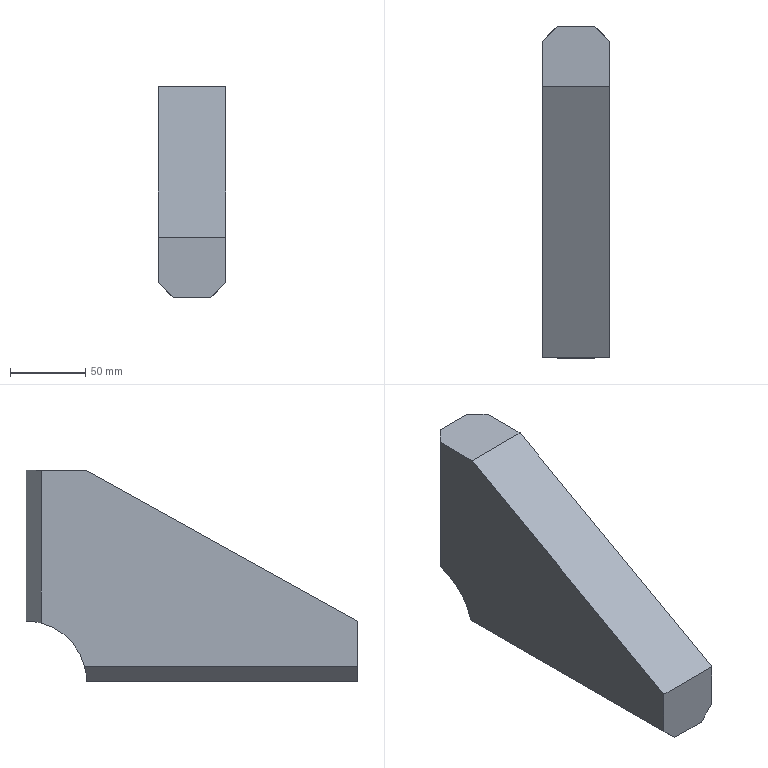Part | SolidWorks | features Chamfer 1, Extrusion 1 | 1 solid | 12 faces | box 45 x 220 x 140 mm | volume 896409 mm3 | plane 11 | cylinder 1 | commonest cylinder face diameters 80 x1
STEP:
#1=CARTESIAN_POINT('',(-22.5,0.,40.));
#2=VERTEX_POINT('',#1);
#3=CARTESIAN_POINT('',(-22.5,0.,10.));
#4=VERTEX_POINT('',#3);
#5=CARTESIAN_POINT('',(-22.5,0.,40.));
#6=DIRECTION('',(0.,0.,-1.));
#7=VECTOR('',#6,1000.);
#8=LINE('',#5,#7);
#9=EDGE_CURVE('',#2,#4,#8,.T.);
#10=ORIENTED_EDGE('',*,*,#9,.T.);
#11=CARTESIAN_POINT('',(-12.5,0.,0.));
#12=VERTEX_POINT('',#11);
#13=CARTESIAN_POINT('',(-12.5,0.,0.));
#14=DIRECTION('',(0.7071,0.,-0.7071));
#15=VECTOR('',#14,1000.);
#16=LINE('',#13,#15);
#17=EDGE_CURVE('',#4,#12,#16,.T.);
#18=ORIENTED_EDGE('',*,*,#17,.T.);
#19=CARTESIAN_POINT('',(12.5,0.,0.));
#20=VERTEX_POINT('',#19);
#21=CARTESIAN_POINT('',(22.5,0.,0.));
#22=DIRECTION('',(-1.,0.,0.));
#23=VECTOR('',#22,1000.);
#24=LINE('',#21,#23);
#25=EDGE_CURVE('',#20,#12,#24,.T.);
#26=ORIENTED_EDGE('',*,*,#25,.F.);
#27=CARTESIAN_POINT('',(22.5,0.,10.));
#28=VERTEX_POINT('',#27);
#29=CARTESIAN_POINT('',(22.5,0.,10.));
#30=DIRECTION('',(0.7071,0.,0.7071));
#31=VECTOR('',#30,1000.);
#32=LINE('',#29,#31);
#33=EDGE_CURVE('',#20,#28,#32,.T.);
#34=ORIENTED_EDGE('',*,*,#33,.T.);
#35=CARTESIAN_POINT('',(22.5,0.,40.));
#36=VERTEX_POINT('',#35);
#37=CARTESIAN_POINT('',(22.5,0.,40.));
#38=DIRECTION('',(0.,0.,-1.));
#39=VECTOR('',#38,1000.);
#40=LINE('',#37,#39);
#41=EDGE_CURVE('',#36,#28,#40,.T.);
#42=ORIENTED_EDGE('',*,*,#41,.F.);
#43=CARTESIAN_POINT('',(22.5,0.,40.));
#44=DIRECTION('',(-1.,0.,0.));
#45=VECTOR('',#44,1000.);
#46=LINE('',#43,#45);
#47=EDGE_CURVE('',#36,#2,#46,.T.);
#48=ORIENTED_EDGE('',*,*,#47,.T.);
#49=EDGE_LOOP('',(#10,#18,#26,#34,#42,#48));
#50=FACE_OUTER_BOUND('',#49,.T.);
#51=CARTESIAN_POINT('',(22.5,0.,40.));
#52=DIRECTION('',(0.,1.,0.));
#53=DIRECTION('',(0.,0.,1.));
#54=AXIS2_PLACEMENT_3D('',#51,#52,#53);
#55=PLANE('',#54);
#56=ADVANCED_FACE('',(#50),#55,.F.);
#57=ORIENTED_EDGE('',*,*,#25,.T.);
#58=CARTESIAN_POINT('',(-12.5,180.,0.));
#59=VERTEX_POINT('',#58);
#60=CARTESIAN_POINT('',(-12.5,0.,0.));
#61=DIRECTION('',(0.,1.,0.));
#62=VECTOR('',#61,1000.);
#63=LINE('',#60,#62);
#64=EDGE_CURVE('',#12,#59,#63,.T.);
#65=ORIENTED_EDGE('',*,*,#64,.T.);
#66=CARTESIAN_POINT('',(12.5,180.,0.));
#67=VERTEX_POINT('',#66);
#68=CARTESIAN_POINT('',(22.5,180.,0.));
#69=DIRECTION('',(-1.,0.,0.));
#70=VECTOR('',#69,1000.);
#71=LINE('',#68,#70);
#72=EDGE_CURVE('',#67,#59,#71,.T.);
#73=ORIENTED_EDGE('',*,*,#72,.F.);
#74=CARTESIAN_POINT('',(12.5,0.,0.));
#75=DIRECTION('',(0.,-1.,0.));
#76=VECTOR('',#75,1000.);
#77=LINE('',#74,#76);
#78=EDGE_CURVE('',#67,#20,#77,.T.);
#79=ORIENTED_EDGE('',*,*,#78,.T.);
#80=EDGE_LOOP('',(#57,#65,#73,#79));
#81=FACE_OUTER_BOUND('',#80,.T.);
#82=CARTESIAN_POINT('',(22.5,0.,0.));
#83=DIRECTION('',(0.,0.,1.));
#84=DIRECTION('',(1.,0.,0.));
#85=AXIS2_PLACEMENT_3D('',#82,#83,#84);
#86=PLANE('',#85);
#87=ADVANCED_FACE('',(#81),#86,.F.);
#88=CARTESIAN_POINT('',(12.5,220.,40.));
#89=VERTEX_POINT('',#88);
#90=CARTESIAN_POINT('',(-12.5,220.,40.));
#91=VERTEX_POINT('',#90);
#92=CARTESIAN_POINT('',(22.5,220.,40.));
#93=DIRECTION('',(-1.,0.,0.));
#94=VECTOR('',#93,1000.);
#95=LINE('',#92,#94);
#96=EDGE_CURVE('',#89,#91,#95,.T.);
#97=ORIENTED_EDGE('',*,*,#96,.F.);
#98=CARTESIAN_POINT('',(22.5,210.,38.73));
#99=VERTEX_POINT('',#98);
#100=CARTESIAN_POINT('',(12.5,220.,40.));
#101=CARTESIAN_POINT('',(15.878,216.622,40.));
#102=CARTESIAN_POINT('',(19.229,213.271,39.574));
#103=CARTESIAN_POINT('',(22.5,210.,38.73));
#104=(BOUNDED_CURVE()B_SPLINE_CURVE(3,(#100,#101,#102,#103),.UNSPECIFIED.,.F.,.F.)B_SPLINE_CURVE_WITH_KNOTS((4,4),(1.571,1.823),.UNSPECIFIED.)CURVE()GEOMETRIC_REPRESENTATION_ITEM()RATIONAL_B_SPLINE_CURVE((1.,0.9947,0.9947,1.))REPRESENTATION_ITEM(''));
#105=EDGE_CURVE('',#89,#99,#104,.T.);
#106=ORIENTED_EDGE('',*,*,#105,.T.);
#107=CARTESIAN_POINT('',(22.5,181.27,10.));
#108=VERTEX_POINT('',#107);
#109=CARTESIAN_POINT('',(22.5,220.,0.));
#110=DIRECTION('',(-1.,0.,0.));
#111=DIRECTION('',(0.,0.,-1.));
#112=AXIS2_PLACEMENT_3D('',#109,#110,#111);
#113=CIRCLE('',#112,40.);
#114=EDGE_CURVE('',#108,#99,#113,.T.);
#115=ORIENTED_EDGE('',*,*,#114,.F.);
#116=CARTESIAN_POINT('',(22.5,181.27,10.));
#117=CARTESIAN_POINT('',(19.229,180.426,6.729));
#118=CARTESIAN_POINT('',(15.878,180.,3.378));
#119=CARTESIAN_POINT('',(12.5,180.,0.));
#120=(BOUNDED_CURVE()B_SPLINE_CURVE(3,(#116,#117,#118,#119),.UNSPECIFIED.,.F.,.F.)B_SPLINE_CURVE_WITH_KNOTS((4,4),(4.46,4.712),.UNSPECIFIED.)CURVE()GEOMETRIC_REPRESENTATION_ITEM()RATIONAL_B_SPLINE_CURVE((1.,0.9947,0.9947,1.))REPRESENTATION_ITEM(''));
#121=EDGE_CURVE('',#108,#67,#120,.T.);
#122=ORIENTED_EDGE('',*,*,#121,.T.);
#123=ORIENTED_EDGE('',*,*,#72,.T.);
#124=CARTESIAN_POINT('',(-22.5,181.27,10.));
#125=VERTEX_POINT('',#124);
#126=CARTESIAN_POINT('',(-12.5,180.,0.));
#127=CARTESIAN_POINT('',(-15.878,180.,3.378));
#128=CARTESIAN_POINT('',(-19.229,180.426,6.729));
#129=CARTESIAN_POINT('',(-22.5,181.27,10.));
#130=(BOUNDED_CURVE()B_SPLINE_CURVE(3,(#126,#127,#128,#129),.UNSPECIFIED.,.F.,.F.)B_SPLINE_CURVE_WITH_KNOTS((4,4),(4.712,4.965),.UNSPECIFIED.)CURVE()GEOMETRIC_REPRESENTATION_ITEM()RATIONAL_B_SPLINE_CURVE((1.,0.9947,0.9947,1.))REPRESENTATION_ITEM(''));
#131=EDGE_CURVE('',#59,#125,#130,.T.);
#132=ORIENTED_EDGE('',*,*,#131,.T.);
#133=CARTESIAN_POINT('',(-22.5,210.,38.73));
#134=VERTEX_POINT('',#133);
#135=CARTESIAN_POINT('',(-22.5,220.,0.));
#136=DIRECTION('',(-1.,0.,0.));
#137=DIRECTION('',(0.,0.,-1.));
#138=AXIS2_PLACEMENT_3D('',#135,#136,#137);
#139=CIRCLE('',#138,40.);
#140=EDGE_CURVE('',#125,#134,#139,.T.);
#141=ORIENTED_EDGE('',*,*,#140,.T.);
#142=CARTESIAN_POINT('',(-22.5,210.,38.73));
#143=CARTESIAN_POINT('',(-19.229,213.271,39.574));
#144=CARTESIAN_POINT('',(-15.878,216.622,40.));
#145=CARTESIAN_POINT('',(-12.5,220.,40.));
#146=(BOUNDED_CURVE()B_SPLINE_CURVE(3,(#142,#143,#144,#145),.UNSPECIFIED.,.F.,.F.)B_SPLINE_CURVE_WITH_KNOTS((4,4),(1.318,1.571),.UNSPECIFIED.)CURVE()GEOMETRIC_REPRESENTATION_ITEM()RATIONAL_B_SPLINE_CURVE((1.,0.9947,0.9947,1.))REPRESENTATION_ITEM(''));
#147=EDGE_CURVE('',#134,#91,#146,.T.);
#148=ORIENTED_EDGE('',*,*,#147,.T.);
#149=EDGE_LOOP('',(#97,#106,#115,#122,#123,#132,#141,#148));
#150=FACE_OUTER_BOUND('',#149,.T.);
#151=CARTESIAN_POINT('',(22.5,220.,0.));
#152=DIRECTION('',(-1.,0.,0.));
#153=DIRECTION('',(0.,0.,1.));
#154=AXIS2_PLACEMENT_3D('',#151,#152,#153);
#155=CYLINDRICAL_SURFACE('',#154,40.);
#156=ADVANCED_FACE('',(#150),#155,.F.);
#157=CARTESIAN_POINT('',(12.5,220.,140.));
#158=VERTEX_POINT('',#157);
#159=CARTESIAN_POINT('',(-12.5,220.,140.));
#160=VERTEX_POINT('',#159);
#161=CARTESIAN_POINT('',(22.5,220.,140.));
#162=DIRECTION('',(-1.,0.,0.));
#163=VECTOR('',#162,1000.);
#164=LINE('',#161,#163);
#165=EDGE_CURVE('',#158,#160,#164,.T.);
#166=ORIENTED_EDGE('',*,*,#165,.F.);
#167=CARTESIAN_POINT('',(12.5,220.,40.));
#168=DIRECTION('',(0.,0.,-1.));
#169=VECTOR('',#168,1000.);
#170=LINE('',#167,#169);
#171=EDGE_CURVE('',#158,#89,#170,.T.);
#172=ORIENTED_EDGE('',*,*,#171,.T.);
#173=ORIENTED_EDGE('',*,*,#96,.T.);
#174=CARTESIAN_POINT('',(-12.5,220.,40.));
#175=DIRECTION('',(0.,0.,1.));
#176=VECTOR('',#175,1000.);
#177=LINE('',#174,#176);
#178=EDGE_CURVE('',#91,#160,#177,.T.);
#179=ORIENTED_EDGE('',*,*,#178,.T.);
#180=EDGE_LOOP('',(#166,#172,#173,#179));
#181=FACE_OUTER_BOUND('',#180,.T.);
#182=CARTESIAN_POINT('',(22.5,220.,40.));
#183=DIRECTION('',(0.,-1.,0.));
#184=DIRECTION('',(0.,0.,-1.));
#185=AXIS2_PLACEMENT_3D('',#182,#183,#184);
#186=PLANE('',#185);
#187=ADVANCED_FACE('',(#181),#186,.F.);
#188=CARTESIAN_POINT('',(22.5,210.,140.));
#189=VERTEX_POINT('',#188);
#190=CARTESIAN_POINT('',(22.5,180.,140.));
#191=VERTEX_POINT('',#190);
#192=CARTESIAN_POINT('',(22.5,220.,140.));
#193=DIRECTION('',(0.,-1.,0.));
#194=VECTOR('',#193,1000.);
#195=LINE('',#192,#194);
#196=EDGE_CURVE('',#189,#191,#195,.T.);
#197=ORIENTED_EDGE('',*,*,#196,.F.);
#198=CARTESIAN_POINT('',(22.5,210.,140.));
#199=DIRECTION('',(-0.7071,0.7071,0.));
#200=VECTOR('',#199,1000.);
#201=LINE('',#198,#200);
#202=EDGE_CURVE('',#189,#158,#201,.T.);
#203=ORIENTED_EDGE('',*,*,#202,.T.);
#204=ORIENTED_EDGE('',*,*,#165,.T.);
#205=CARTESIAN_POINT('',(-22.5,210.,140.));
#206=VERTEX_POINT('',#205);
#207=CARTESIAN_POINT('',(-12.5,220.,140.));
#208=DIRECTION('',(-0.7071,-0.7071,0.));
#209=VECTOR('',#208,1000.);
#210=LINE('',#207,#209);
#211=EDGE_CURVE('',#160,#206,#210,.T.);
#212=ORIENTED_EDGE('',*,*,#211,.T.);
#213=CARTESIAN_POINT('',(-22.5,180.,140.));
#214=VERTEX_POINT('',#213);
#215=CARTESIAN_POINT('',(-22.5,220.,140.));
#216=DIRECTION('',(0.,-1.,0.));
#217=VECTOR('',#216,1000.);
#218=LINE('',#215,#217);
#219=EDGE_CURVE('',#206,#214,#218,.T.);
#220=ORIENTED_EDGE('',*,*,#219,.T.);
#221=CARTESIAN_POINT('',(22.5,180.,140.));
#222=DIRECTION('',(-1.,0.,0.));
#223=VECTOR('',#222,1000.);
#224=LINE('',#221,#223);
#225=EDGE_CURVE('',#191,#214,#224,.T.);
#226=ORIENTED_EDGE('',*,*,#225,.F.);
#227=EDGE_LOOP('',(#197,#203,#204,#212,#220,#226));
#228=FACE_OUTER_BOUND('',#227,.T.);
#229=CARTESIAN_POINT('',(22.5,220.,140.));
#230=DIRECTION('',(0.,0.,-1.));
#231=DIRECTION('',(-1.,0.,0.));
#232=AXIS2_PLACEMENT_3D('',#229,#230,#231);
#233=PLANE('',#232);
#234=ADVANCED_FACE('',(#228),#233,.F.);
#235=CARTESIAN_POINT('',(-22.5,180.,140.));
#236=DIRECTION('',(0.,-0.8742,-0.4856));
#237=VECTOR('',#236,1000.);
#238=LINE('',#235,#237);
#239=EDGE_CURVE('',#214,#2,#238,.T.);
#240=ORIENTED_EDGE('',*,*,#239,.T.);
#241=ORIENTED_EDGE('',*,*,#47,.F.);
#242=CARTESIAN_POINT('',(22.5,180.,140.));
#243=DIRECTION('',(0.,-0.8742,-0.4856));
#244=VECTOR('',#243,1000.);
#245=LINE('',#242,#244);
#246=EDGE_CURVE('',#191,#36,#245,.T.);
#247=ORIENTED_EDGE('',*,*,#246,.F.);
#248=ORIENTED_EDGE('',*,*,#225,.T.);
#249=EDGE_LOOP('',(#240,#241,#247,#248));
#250=FACE_OUTER_BOUND('',#249,.T.);
#251=CARTESIAN_POINT('',(22.5,180.,140.));
#252=DIRECTION('',(0.,0.4856,-0.8742));
#253=DIRECTION('',(0.,0.8742,0.4856));
#254=AXIS2_PLACEMENT_3D('',#251,#252,#253);
#255=PLANE('',#254);
#256=ADVANCED_FACE('',(#250),#255,.F.);
#257=ORIENTED_EDGE('',*,*,#114,.T.);
#258=CARTESIAN_POINT('',(22.5,210.,140.));
#259=DIRECTION('',(0.,0.,1.));
#260=VECTOR('',#259,1000.);
#261=LINE('',#258,#260);
#262=EDGE_CURVE('',#99,#189,#261,.T.);
#263=ORIENTED_EDGE('',*,*,#262,.T.);
#264=ORIENTED_EDGE('',*,*,#196,.T.);
#265=ORIENTED_EDGE('',*,*,#246,.T.);
#266=ORIENTED_EDGE('',*,*,#41,.T.);
#267=CARTESIAN_POINT('',(22.5,180.,10.));
#268=DIRECTION('',(0.,1.,0.));
#269=VECTOR('',#268,1000.);
#270=LINE('',#267,#269);
#271=EDGE_CURVE('',#28,#108,#270,.T.);
#272=ORIENTED_EDGE('',*,*,#271,.T.);
#273=EDGE_LOOP('',(#257,#263,#264,#265,#266,#272));
#274=FACE_OUTER_BOUND('',#273,.T.);
#275=CARTESIAN_POINT('',(22.5,220.,0.));
#276=DIRECTION('',(1.,0.,0.));
#277=DIRECTION('',(0.,0.,-1.));
#278=AXIS2_PLACEMENT_3D('',#275,#276,#277);
#279=PLANE('',#278);
#280=ADVANCED_FACE('',(#274),#279,.T.);
#281=ORIENTED_EDGE('',*,*,#219,.F.);
#282=CARTESIAN_POINT('',(-22.5,210.,0.));
#283=DIRECTION('',(0.,0.,-1.));
#284=VECTOR('',#283,1000.);
#285=LINE('',#282,#284);
#286=EDGE_CURVE('',#206,#134,#285,.T.);
#287=ORIENTED_EDGE('',*,*,#286,.T.);
#288=ORIENTED_EDGE('',*,*,#140,.F.);
#289=CARTESIAN_POINT('',(-22.5,220.,10.));
#290=DIRECTION('',(0.,-1.,0.));
#291=VECTOR('',#290,1000.);
#292=LINE('',#289,#291);
#293=EDGE_CURVE('',#125,#4,#292,.T.);
#294=ORIENTED_EDGE('',*,*,#293,.T.);
#295=ORIENTED_EDGE('',*,*,#9,.F.);
#296=ORIENTED_EDGE('',*,*,#239,.F.);
#297=EDGE_LOOP('',(#281,#287,#288,#294,#295,#296));
#298=FACE_OUTER_BOUND('',#297,.T.);
#299=CARTESIAN_POINT('',(-22.5,220.,0.));
#300=DIRECTION('',(1.,0.,0.));
#301=DIRECTION('',(0.,0.,-1.));
#302=AXIS2_PLACEMENT_3D('',#299,#300,#301);
#303=PLANE('',#302);
#304=ADVANCED_FACE('',(#298),#303,.F.);
#305=ORIENTED_EDGE('',*,*,#105,.F.);
#306=ORIENTED_EDGE('',*,*,#171,.F.);
#307=ORIENTED_EDGE('',*,*,#202,.F.);
#308=ORIENTED_EDGE('',*,*,#262,.F.);
#309=EDGE_LOOP('',(#305,#306,#307,#308));
#310=FACE_OUTER_BOUND('',#309,.T.);
#311=CARTESIAN_POINT('',(22.5,210.,0.));
#312=DIRECTION('',(0.7071,0.7071,0.));
#313=DIRECTION('',(0.,0.,-1.));
#314=AXIS2_PLACEMENT_3D('',#311,#312,#313);
#315=PLANE('',#314);
#316=ADVANCED_FACE('',(#310),#315,.T.);
#317=ORIENTED_EDGE('',*,*,#147,.F.);
#318=ORIENTED_EDGE('',*,*,#286,.F.);
#319=ORIENTED_EDGE('',*,*,#211,.F.);
#320=ORIENTED_EDGE('',*,*,#178,.F.);
#321=EDGE_LOOP('',(#317,#318,#319,#320));
#322=FACE_OUTER_BOUND('',#321,.T.);
#323=CARTESIAN_POINT('',(-12.5,220.,40.));
#324=DIRECTION('',(0.7071,-0.7071,0.));
#325=DIRECTION('',(0.,0.,1.));
#326=AXIS2_PLACEMENT_3D('',#323,#324,#325);
#327=PLANE('',#326);
#328=ADVANCED_FACE('',(#322),#327,.F.);
#329=ORIENTED_EDGE('',*,*,#17,.F.);
#330=ORIENTED_EDGE('',*,*,#293,.F.);
#331=ORIENTED_EDGE('',*,*,#131,.F.);
#332=ORIENTED_EDGE('',*,*,#64,.F.);
#333=EDGE_LOOP('',(#329,#330,#331,#332));
#334=FACE_OUTER_BOUND('',#333,.T.);
#335=CARTESIAN_POINT('',(-12.5,0.,0.));
#336=DIRECTION('',(0.7071,0.,0.7071));
#337=DIRECTION('',(0.,1.,0.));
#338=AXIS2_PLACEMENT_3D('',#335,#336,#337);
#339=PLANE('',#338);
#340=ADVANCED_FACE('',(#334),#339,.F.);
#341=ORIENTED_EDGE('',*,*,#33,.F.);
#342=ORIENTED_EDGE('',*,*,#78,.F.);
#343=ORIENTED_EDGE('',*,*,#121,.F.);
#344=ORIENTED_EDGE('',*,*,#271,.F.);
#345=EDGE_LOOP('',(#341,#342,#343,#344));
#346=FACE_OUTER_BOUND('',#345,.T.);
#347=CARTESIAN_POINT('',(22.5,220.,10.));
#348=DIRECTION('',(0.7071,0.,-0.7071));
#349=DIRECTION('',(0.,-1.,0.));
#350=AXIS2_PLACEMENT_3D('',#347,#348,#349);
#351=PLANE('',#350);
#352=ADVANCED_FACE('',(#346),#351,.T.);
#353=CLOSED_SHELL('',(#56,#87,#156,#187,#234,#256,#280,#304,#316,#328,#340,#352));
#354=MANIFOLD_SOLID_BREP('',#353);
#355=CARTESIAN_POINT('',(0.,0.,0.));
#356=DIRECTION('',(0.,0.,1.));
#357=DIRECTION('',(1.,0.,0.));
#358=AXIS2_PLACEMENT_3D('',#355,#356,#357);
#359=(LENGTH_UNIT()NAMED_UNIT(*)SI_UNIT(.MILLI.,.METRE.));
#360=UNCERTAINTY_MEASURE_WITH_UNIT(LENGTH_MEASURE(0.00001),#359,'','');
#361=(NAMED_UNIT(*)PLANE_ANGLE_UNIT()SI_UNIT($,.RADIAN.));
#362=(NAMED_UNIT(*)SI_UNIT($,.STERADIAN.)SOLID_ANGLE_UNIT());
#363=(GEOMETRIC_REPRESENTATION_CONTEXT(3)GLOBAL_UNCERTAINTY_ASSIGNED_CONTEXT((#360))GLOBAL_UNIT_ASSIGNED_CONTEXT((#359,#361,#362))REPRESENTATION_CONTEXT('',''));
#364=ADVANCED_BREP_SHAPE_REPRESENTATION('',(#354,#358),#363);